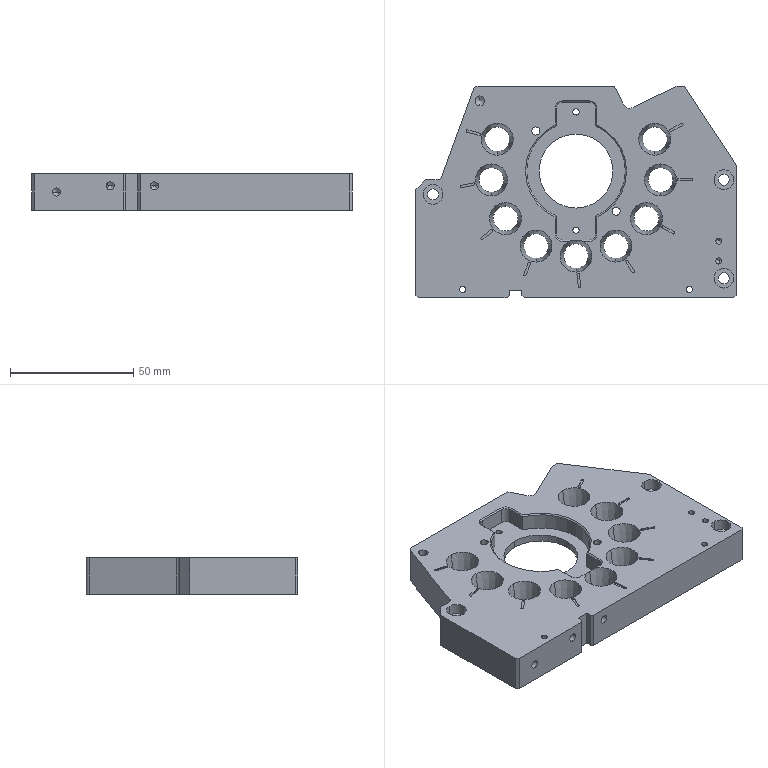NC program | NX | posted with a generic post | part box 130 x 86 x 15 mm
Lines 3061 to 5031 of 5031, first 1542 of 1963 lines:
(FLOOR_WALL_1_COPY_COPY , TOOL : D6JING)
N6120 T16 M6
N6122 G54
N6124 G17 G0 G90 X-5.595 Y18.197 B0. C0. S7500 M3
N6126 G43 Z30. H16
N6128 Z-3.9
N6130 G94 G1 X-9.7 Z-5. F1000.
N6132 X26.7 F1200.
N6134 Y15.397
N6136 X-9.7
N6138 Y12.597
N6140 X26.7
N6142 Y9.798
N6144 X-9.7
N6146 Y6.998
N6148 X26.7
N6150 Y4.198
N6152 X-9.7
N6154 Y1.398
N6156 X26.7
N6158 Y-1.401
N6160 X-9.7
N6162 Y-4.201
N6164 X26.7
N6166 Y-7.001
N6168 X-9.7
N6170 Y-9.801
N6172 X26.7
N6174 Y-12.6
N6176 X-9.7
N6178 Y-15.4
N6180 X26.7
N6182 Y-18.2
N6184 X-9.7
N6186 X-9.
N6188 X-10. F1000.
N6190 Y-18.5 F1200.
N6192 X27.
N6194 Y18.5
N6196 X-10.
N6198 Y-18.2
N6200 X-9.
N6202 Y-17.5
N6204 Z-4.
N6206 G0 Z30.
N6208 M5
(ZLEVEL_PROFILE_1_COPY_COPY , TOOL : D4)
N6210 T17 M6
N6212 G54
N6214 G17 G0 G90 X-10.2 Y-15.91 B0. C0. S6500 M3
N6216 G43 Z30. H17
N6218 Z-0.1
N6220 G94 G1 X-10.8 Y-16.257 F1650.
N6222 G3 X-11. Y-16.603 R0.4
N6224 G1 Y-19.
N6226 G3 X-10.5 Y-19.5 R0.5
N6228 G1 X-8.103
N6230 G3 X-7.757 Y-19.3 R0.4
N6232 G1 X-7.41 Y-18.7
N6234 G0 X-10.2 Y-15.91 Z-0.2
N6236 G1 X-10.8 Y-16.257
N6238 G3 X-11. Y-16.603 R0.4
N6240 G1 Y-19.
N6242 G3 X-10.5 Y-19.5 R0.5
N6244 G1 X-8.103
N6246 G3 X-7.757 Y-19.3 R0.4
N6248 G1 X-7.41 Y-18.7
N6250 G0 X-10.2 Y-15.91 Z-0.3
N6252 G1 X-10.8 Y-16.257
N6254 G3 X-11. Y-16.603 R0.4
N6256 G1 Y-19.
N6258 G3 X-10.5 Y-19.5 R0.5
N6260 G1 X-8.103
N6262 G3 X-7.757 Y-19.3 R0.4
N6264 G1 X-7.41 Y-18.7
N6266 G0 X-10.2 Y-15.91 Z-0.4
N6268 G1 X-10.8 Y-16.257
N6270 G3 X-11. Y-16.603 R0.4
N6272 G1 Y-19.
N6274 G3 X-10.5 Y-19.5 R0.5
N6276 G1 X-8.103
N6278 G3 X-7.757 Y-19.3 R0.4
N6280 G1 X-7.41 Y-18.7
N6282 G0 X-10.2 Y-15.91 Z-0.5
N6284 G1 X-10.8 Y-16.257
N6286 G3 X-11. Y-16.603 R0.4
N6288 G1 Y-19.
N6290 G3 X-10.5 Y-19.5 R0.5
N6292 G1 X-8.103
N6294 G3 X-7.757 Y-19.3 R0.4
N6296 G1 X-7.41 Y-18.7
N6298 G0 X-10.2 Y-15.91 Z-0.6
N6300 G1 X-10.8 Y-16.257
N6302 G3 X-11. Y-16.603 R0.4
N6304 G1 Y-19.
N6306 G3 X-10.5 Y-19.5 R0.5
N6308 G1 X-8.103
N6310 G3 X-7.757 Y-19.3 R0.4
N6312 G1 X-7.41 Y-18.7
N6314 G0 X-10.2 Y-15.91 Z-0.7
N6316 G1 X-10.8 Y-16.257
N6318 G3 X-11. Y-16.603 R0.4
N6320 G1 Y-19.
N6322 G3 X-10.5 Y-19.5 R0.5
N6324 G1 X-8.103
N6326 G3 X-7.757 Y-19.3 R0.4
N6328 G1 X-7.41 Y-18.7
N6330 G0 X-10.2 Y-15.91 Z-0.8
N6332 G1 X-10.8 Y-16.257
N6334 G3 X-11. Y-16.603 R0.4
N6336 G1 Y-19.
N6338 G3 X-10.5 Y-19.5 R0.5
N6340 G1 X-8.103
N6342 G3 X-7.757 Y-19.3 R0.4
N6344 G1 X-7.41 Y-18.7
N6346 G0 X-10.2 Y-15.91 Z-0.9
N6348 G1 X-10.8 Y-16.257
N6350 G3 X-11. Y-16.603 R0.4
N6352 G1 Y-19.
N6354 G3 X-10.5 Y-19.5 R0.5
N6356 G1 X-8.103
N6358 G3 X-7.757 Y-19.3 R0.4
N6360 G1 X-7.41 Y-18.7
N6362 G0 X-10.2 Y-15.91 Z-1.
N6364 G1 X-10.8 Y-16.257
N6366 G3 X-11. Y-16.603 R0.4
N6368 G1 Y-19.
N6370 G3 X-10.5 Y-19.5 R0.5
N6372 G1 X-8.103
N6374 G3 X-7.757 Y-19.3 R0.4
N6376 G1 X-7.41 Y-18.7
N6378 G0 X-10.2 Y-15.91 Z-1.1
N6380 G1 X-10.8 Y-16.257
N6382 G3 X-11. Y-16.603 R0.4
N6384 G1 Y-19.
N6386 G3 X-10.5 Y-19.5 R0.5
N6388 G1 X-8.103
N6390 G3 X-7.757 Y-19.3 R0.4
N6392 G1 X-7.41 Y-18.7
N6394 G0 X-10.2 Y-15.91 Z-1.2
N6396 G1 X-10.8 Y-16.257
N6398 G3 X-11. Y-16.603 R0.4
N6400 G1 Y-19.
N6402 G3 X-10.5 Y-19.5 R0.5
N6404 G1 X-8.103
N6406 G3 X-7.757 Y-19.3 R0.4
N6408 G1 X-7.41 Y-18.7
N6410 G0 X-10.2 Y-15.91 Z-1.3
N6412 G1 X-10.8 Y-16.257
N6414 G3 X-11. Y-16.603 R0.4
N6416 G1 Y-19.
N6418 G3 X-10.5 Y-19.5 R0.5
N6420 G1 X-8.103
N6422 G3 X-7.757 Y-19.3 R0.4
N6424 G1 X-7.41 Y-18.7
N6426 G0 X-10.2 Y-15.91 Z-1.4
N6428 G1 X-10.8 Y-16.257
N6430 G3 X-11. Y-16.603 R0.4
N6432 G1 Y-19.
N6434 G3 X-10.5 Y-19.5 R0.5
N6436 G1 X-8.103
N6438 G3 X-7.757 Y-19.3 R0.4
N6440 G1 X-7.41 Y-18.7
N6442 G0 X-10.2 Y-15.91 Z-1.5
N6444 G1 X-10.8 Y-16.257
N6446 G3 X-11. Y-16.603 R0.4
N6448 G1 Y-19.
N6450 G3 X-10.5 Y-19.5 R0.5
N6452 G1 X-8.103
N6454 G3 X-7.757 Y-19.3 R0.4
N6456 G1 X-7.41 Y-18.7
N6458 G0 X-10.2 Y-15.91 Z-1.6
N6460 G1 X-10.8 Y-16.257
N6462 G3 X-11. Y-16.603 R0.4
N6464 G1 Y-19.
N6466 G3 X-10.5 Y-19.5 R0.5
N6468 G1 X-8.103
N6470 G3 X-7.757 Y-19.3 R0.4
N6472 G1 X-7.41 Y-18.7
N6474 G0 X-10.2 Y-15.91 Z-1.7
N6476 G1 X-10.8 Y-16.257
N6478 G3 X-11. Y-16.603 R0.4
N6480 G1 Y-19.
N6482 G3 X-10.5 Y-19.5 R0.5
N6484 G1 X-8.103
N6486 G3 X-7.757 Y-19.3 R0.4
N6488 G1 X-7.41 Y-18.7
N6490 G0 X-10.2 Y-15.91 Z-1.8
N6492 G1 X-10.8 Y-16.257
N6494 G3 X-11. Y-16.603 R0.4
N6496 G1 Y-19.
N6498 G3 X-10.5 Y-19.5 R0.5
N6500 G1 X-8.103
N6502 G3 X-7.757 Y-19.3 R0.4
N6504 G1 X-7.41 Y-18.7
N6506 G0 X-10.2 Y-15.91 Z-1.9
N6508 G1 X-10.8 Y-16.257
N6510 G3 X-11. Y-16.603 R0.4
N6512 G1 Y-19.
N6514 G3 X-10.5 Y-19.5 R0.5
N6516 G1 X-8.103
N6518 G3 X-7.757 Y-19.3 R0.4
N6520 G1 X-7.41 Y-18.7
N6522 G0 X-10.2 Y-15.91 Z-2.
N6524 G1 X-10.8 Y-16.257
N6526 G3 X-11. Y-16.603 R0.4
N6528 G1 Y-19.
N6530 G3 X-10.5 Y-19.5 R0.5
N6532 G1 X-8.103
N6534 G3 X-7.757 Y-19.3 R0.4
N6536 G1 X-7.41 Y-18.7
N6538 G0 X-10.2 Y-15.91 Z-2.1
N6540 G1 X-10.8 Y-16.257
N6542 G3 X-11. Y-16.603 R0.4
N6544 G1 Y-19.
N6546 G3 X-10.5 Y-19.5 R0.5
N6548 G1 X-8.103
N6550 G3 X-7.757 Y-19.3 R0.4
N6552 G1 X-7.41 Y-18.7
N6554 G0 X-10.2 Y-15.91 Z-2.2
N6556 G1 X-10.8 Y-16.257
N6558 G3 X-11. Y-16.603 R0.4
N6560 G1 Y-19.
N6562 G3 X-10.5 Y-19.5 R0.5
N6564 G1 X-8.103
N6566 G3 X-7.757 Y-19.3 R0.4
N6568 G1 X-7.41 Y-18.7
N6570 G0 X-10.2 Y-15.91 Z-2.3
N6572 G1 X-10.8 Y-16.257
N6574 G3 X-11. Y-16.603 R0.4
N6576 G1 Y-19.
N6578 G3 X-10.5 Y-19.5 R0.5
N6580 G1 X-8.103
N6582 G3 X-7.757 Y-19.3 R0.4
N6584 G1 X-7.41 Y-18.7
N6586 G0 X-10.2 Y-15.91 Z-2.4
N6588 G1 X-10.8 Y-16.257
N6590 G3 X-11. Y-16.603 R0.4
N6592 G1 Y-19.
N6594 G3 X-10.5 Y-19.5 R0.5
N6596 G1 X-8.103
N6598 G3 X-7.757 Y-19.3 R0.4
N6600 G1 X-7.41 Y-18.7
N6602 G0 X-10.2 Y-15.91 Z-2.5
N6604 G1 X-10.8 Y-16.257
N6606 G3 X-11. Y-16.603 R0.4
N6608 G1 Y-19.
N6610 G3 X-10.5 Y-19.5 R0.5
N6612 G1 X-8.103
N6614 G3 X-7.757 Y-19.3 R0.4
N6616 G1 X-7.41 Y-18.7
N6618 G0 X-10.2 Y-15.91 Z-2.6
N6620 G1 X-10.8 Y-16.257
N6622 G3 X-11. Y-16.603 R0.4
N6624 G1 Y-19.
N6626 G3 X-10.5 Y-19.5 R0.5
N6628 G1 X-8.103
N6630 G3 X-7.757 Y-19.3 R0.4
N6632 G1 X-7.41 Y-18.7
N6634 G0 X-10.2 Y-15.91 Z-2.7
N6636 G1 X-10.8 Y-16.257
N6638 G3 X-11. Y-16.603 R0.4
N6640 G1 Y-19.
N6642 G3 X-10.5 Y-19.5 R0.5
N6644 G1 X-8.103
N6646 G3 X-7.757 Y-19.3 R0.4
N6648 G1 X-7.41 Y-18.7
N6650 G0 X-10.2 Y-15.91 Z-2.8
N6652 G1 X-10.8 Y-16.257
N6654 G3 X-11. Y-16.603 R0.4
N6656 G1 Y-19.
N6658 G3 X-10.5 Y-19.5 R0.5
N6660 G1 X-8.103
N6662 G3 X-7.757 Y-19.3 R0.4
N6664 G1 X-7.41 Y-18.7
N6666 G0 X-10.2 Y-15.91 Z-2.9
N6668 G1 X-10.8 Y-16.257
N6670 G3 X-11. Y-16.603 R0.4
N6672 G1 Y-19.
N6674 G3 X-10.5 Y-19.5 R0.5
N6676 G1 X-8.103
N6678 G3 X-7.757 Y-19.3 R0.4
N6680 G1 X-7.41 Y-18.7
N6682 G0 X-10.2 Y-15.91 Z-3.
N6684 G1 X-10.8 Y-16.257
N6686 G3 X-11. Y-16.603 R0.4
N6688 G1 Y-19.
N6690 G3 X-10.5 Y-19.5 R0.5
N6692 G1 X-8.103
N6694 G3 X-7.757 Y-19.3 R0.4
N6696 G1 X-7.41 Y-18.7
N6698 G0 X-10.2 Y-15.91 Z-3.1
N6700 G1 X-10.8 Y-16.257
N6702 G3 X-11. Y-16.603 R0.4
N6704 G1 Y-19.
N6706 G3 X-10.5 Y-19.5 R0.5
N6708 G1 X-8.103
N6710 G3 X-7.757 Y-19.3 R0.4
N6712 G1 X-7.41 Y-18.7
N6714 G0 X-10.2 Y-15.91 Z-3.2
N6716 G1 X-10.8 Y-16.257
N6718 G3 X-11. Y-16.603 R0.4
N6720 G1 Y-19.
N6722 G3 X-10.5 Y-19.5 R0.5
N6724 G1 X-8.103
N6726 G3 X-7.757 Y-19.3 R0.4
N6728 G1 X-7.41 Y-18.7
N6730 G0 X-10.2 Y-15.91 Z-3.3
N6732 G1 X-10.8 Y-16.257
N6734 G3 X-11. Y-16.603 R0.4
N6736 G1 Y-19.
N6738 G3 X-10.5 Y-19.5 R0.5
N6740 G1 X-8.103
N6742 G3 X-7.757 Y-19.3 R0.4
N6744 G1 X-7.41 Y-18.7
N6746 G0 X-10.2 Y-15.91 Z-3.4
N6748 G1 X-10.8 Y-16.257
N6750 G3 X-11. Y-16.603 R0.4
N6752 G1 Y-19.
N6754 G3 X-10.5 Y-19.5 R0.5
N6756 G1 X-8.103
N6758 G3 X-7.757 Y-19.3 R0.4
N6760 G1 X-7.41 Y-18.7
N6762 G0 X-10.2 Y-15.91 Z-3.5
N6764 G1 X-10.8 Y-16.257
N6766 G3 X-11. Y-16.603 R0.4
N6768 G1 Y-19.
N6770 G3 X-10.5 Y-19.5 R0.5
N6772 G1 X-8.103
N6774 G3 X-7.757 Y-19.3 R0.4
N6776 G1 X-7.41 Y-18.7
N6778 G0 X-10.2 Y-15.91 Z-3.6
N6780 G1 X-10.8 Y-16.257
N6782 G3 X-11. Y-16.603 R0.4
N6784 G1 Y-19.
N6786 G3 X-10.5 Y-19.5 R0.5
N6788 G1 X-8.103
N6790 G3 X-7.757 Y-19.3 R0.4
N6792 G1 X-7.41 Y-18.7
N6794 G0 X-10.2 Y-15.91 Z-3.7
N6796 G1 X-10.8 Y-16.257
N6798 G3 X-11. Y-16.603 R0.4
N6800 G1 Y-19.
N6802 G3 X-10.5 Y-19.5 R0.5
N6804 G1 X-8.103
N6806 G3 X-7.757 Y-19.3 R0.4
N6808 G1 X-7.41 Y-18.7
N6810 G0 X-10.2 Y-15.91 Z-3.8
N6812 G1 X-10.8 Y-16.257
N6814 G3 X-11. Y-16.603 R0.4
N6816 G1 Y-19.
N6818 G3 X-10.5 Y-19.5 R0.5
N6820 G1 X-8.103
N6822 G3 X-7.757 Y-19.3 R0.4
N6824 G1 X-7.41 Y-18.7
N6826 G0 X-10.2 Y-15.91 Z-3.9
N6828 G1 X-10.8 Y-16.257
N6830 G3 X-11. Y-16.603 R0.4
N6832 G1 Y-19.
N6834 G3 X-10.5 Y-19.5 R0.5
N6836 G1 X-8.103
N6838 G3 X-7.757 Y-19.3 R0.4
N6840 G1 X-7.41 Y-18.7
N6842 G0 X-10.2 Y-15.91 Z-4.
N6844 G1 X-10.8 Y-16.257
N6846 G3 X-11. Y-16.603 R0.4
N6848 G1 Y-19.
N6850 G3 X-10.5 Y-19.5 R0.5
N6852 G1 X-8.103
N6854 G3 X-7.757 Y-19.3 R0.4
N6856 G1 X-7.41 Y-18.7
N6858 G0 X-10.2 Y-15.91 Z-4.1
N6860 G1 X-10.8 Y-16.257
N6862 G3 X-11. Y-16.603 R0.4
N6864 G1 Y-19.
N6866 G3 X-10.5 Y-19.5 R0.5
N6868 G1 X-8.103
N6870 G3 X-7.757 Y-19.3 R0.4
N6872 G1 X-7.41 Y-18.7
N6874 G0 X-10.2 Y-15.91 Z-4.2
N6876 G1 X-10.8 Y-16.257
N6878 G3 X-11. Y-16.603 R0.4
N6880 G1 Y-19.
N6882 G3 X-10.5 Y-19.5 R0.5
N6884 G1 X-8.103
N6886 G3 X-7.757 Y-19.3 R0.4
N6888 G1 X-7.41 Y-18.7
N6890 G0 X-10.2 Y-15.91 Z-4.3
N6892 G1 X-10.8 Y-16.257
N6894 G3 X-11. Y-16.603 R0.4
N6896 G1 Y-19.
N6898 G3 X-10.5 Y-19.5 R0.5
N6900 G1 X-8.103
N6902 G3 X-7.757 Y-19.3 R0.4
N6904 G1 X-7.41 Y-18.7
N6906 G0 X-10.2 Y-15.91 Z-4.4
N6908 G1 X-10.8 Y-16.257
N6910 G3 X-11. Y-16.603 R0.4
N6912 G1 Y-19.
N6914 G3 X-10.5 Y-19.5 R0.5
N6916 G1 X-8.103
N6918 G3 X-7.757 Y-19.3 R0.4
N6920 G1 X-7.41 Y-18.7
N6922 G0 X-10.2 Y-15.91 Z-4.5
N6924 G1 X-10.8 Y-16.257
N6926 G3 X-11. Y-16.603 R0.4
N6928 G1 Y-19.
N6930 G3 X-10.5 Y-19.5 R0.5
N6932 G1 X-8.103
N6934 G3 X-7.757 Y-19.3 R0.4
N6936 G1 X-7.41 Y-18.7
N6938 G0 X-10.2 Y-15.91 Z-4.6
N6940 G1 X-10.8 Y-16.257
N6942 G3 X-11. Y-16.603 R0.4
N6944 G1 Y-19.
N6946 G3 X-10.5 Y-19.5 R0.5
N6948 G1 X-8.103
N6950 G3 X-7.757 Y-19.3 R0.4
N6952 G1 X-7.41 Y-18.7
N6954 G0 X-10.2 Y-15.91 Z-4.7
N6956 G1 X-10.8 Y-16.257
N6958 G3 X-11. Y-16.603 R0.4
N6960 G1 Y-19.
N6962 G3 X-10.5 Y-19.5 R0.5
N6964 G1 X-8.103
N6966 G3 X-7.757 Y-19.3 R0.4
N6968 G1 X-7.41 Y-18.7
N6970 G0 X-10.2 Y-15.91 Z-4.8
N6972 G1 X-10.8 Y-16.257
N6974 G3 X-11. Y-16.603 R0.4
N6976 G1 Y-19.
N6978 G3 X-10.5 Y-19.5 R0.5
N6980 G1 X-8.103
N6982 G3 X-7.757 Y-19.3 R0.4
N6984 G1 X-7.41 Y-18.7
N6986 G0 X-10.2 Y-15.91 Z-4.9
N6988 G1 X-10.8 Y-16.257
N6990 G3 X-11. Y-16.603 R0.4
N6992 G1 Y-19.
N6994 G3 X-10.5 Y-19.5 R0.5
N6996 G1 X-8.103
N6998 G3 X-7.757 Y-19.3 R0.4
N7000 G1 X-7.41 Y-18.7
N7002 G0 X-10.2 Y-15.91 Z-5.
N7004 G1 X-10.8 Y-16.257
N7006 G3 X-11. Y-16.603 R0.4
N7008 G1 Y-19.
N7010 G3 X-10.5 Y-19.5 R0.5
N7012 G1 X-8.103
N7014 G3 X-7.757 Y-19.3 R0.4
N7016 G1 X-7.41 Y-18.7
N7018 G0 Z30.
N7020 X24.41
N7022 Z-0.1
N7024 G1 X24.757 Y-19.3
N7026 G3 X25.103 Y-19.5 R0.4
N7028 G1 X27.5
N7030 G3 X28. Y-19. R0.5
N7032 G1 Y-16.603
N7034 G3 X27.8 Y-16.257 R0.4
N7036 G1 X27.2 Y-15.91
N7038 G0 X24.41 Y-18.7 Z-0.2
N7040 G1 X24.757 Y-19.3
N7042 G3 X25.103 Y-19.5 R0.4
N7044 G1 X27.5
N7046 G3 X28. Y-19. R0.5
N7048 G1 Y-16.603
N7050 G3 X27.8 Y-16.257 R0.4
N7052 G1 X27.2 Y-15.91
N7054 G0 X24.41 Y-18.7 Z-0.3
N7056 G1 X24.757 Y-19.3
N7058 G3 X25.103 Y-19.5 R0.4
N7060 G1 X27.5
N7062 G3 X28. Y-19. R0.5
N7064 G1 Y-16.603
N7066 G3 X27.8 Y-16.257 R0.4
N7068 G1 X27.2 Y-15.91
N7070 G0 X24.41 Y-18.7 Z-0.4
N7072 G1 X24.757 Y-19.3
N7074 G3 X25.103 Y-19.5 R0.4
N7076 G1 X27.5
N7078 G3 X28. Y-19. R0.5
N7080 G1 Y-16.603
N7082 G3 X27.8 Y-16.257 R0.4
N7084 G1 X27.2 Y-15.91
N7086 G0 X24.41 Y-18.7 Z-0.5
N7088 G1 X24.757 Y-19.3
N7090 G3 X25.103 Y-19.5 R0.4
N7092 G1 X27.5
N7094 G3 X28. Y-19. R0.5
N7096 G1 Y-16.603
N7098 G3 X27.8 Y-16.257 R0.4
N7100 G1 X27.2 Y-15.91
N7102 G0 X24.41 Y-18.7 Z-0.6
N7104 G1 X24.757 Y-19.3
N7106 G3 X25.103 Y-19.5 R0.4
N7108 G1 X27.5
N7110 G3 X28. Y-19. R0.5
N7112 G1 Y-16.603
N7114 G3 X27.8 Y-16.257 R0.4
N7116 G1 X27.2 Y-15.91
N7118 G0 X24.41 Y-18.7 Z-0.7
N7120 G1 X24.757 Y-19.3
N7122 G3 X25.103 Y-19.5 R0.4
N7124 G1 X27.5
N7126 G3 X28. Y-19. R0.5
N7128 G1 Y-16.603
N7130 G3 X27.8 Y-16.257 R0.4
N7132 G1 X27.2 Y-15.91
N7134 G0 X24.41 Y-18.7 Z-0.8
N7136 G1 X24.757 Y-19.3
N7138 G3 X25.103 Y-19.5 R0.4
N7140 G1 X27.5
N7142 G3 X28. Y-19. R0.5
N7144 G1 Y-16.603
N7146 G3 X27.8 Y-16.257 R0.4
N7148 G1 X27.2 Y-15.91
N7150 G0 X24.41 Y-18.7 Z-0.9
N7152 G1 X24.757 Y-19.3
N7154 G3 X25.103 Y-19.5 R0.4
N7156 G1 X27.5
N7158 G3 X28. Y-19. R0.5
N7160 G1 Y-16.603
N7162 G3 X27.8 Y-16.257 R0.4
N7164 G1 X27.2 Y-15.91
N7166 G0 X24.41 Y-18.7 Z-1.
N7168 G1 X24.757 Y-19.3
N7170 G3 X25.103 Y-19.5 R0.4
N7172 G1 X27.5
N7174 G3 X28. Y-19. R0.5
N7176 G1 Y-16.603
N7178 G3 X27.8 Y-16.257 R0.4
N7180 G1 X27.2 Y-15.91
N7182 G0 X24.41 Y-18.7 Z-1.1
N7184 G1 X24.757 Y-19.3
N7186 G3 X25.103 Y-19.5 R0.4
N7188 G1 X27.5
N7190 G3 X28. Y-19. R0.5
N7192 G1 Y-16.603
N7194 G3 X27.8 Y-16.257 R0.4
N7196 G1 X27.2 Y-15.91
N7198 G0 X24.41 Y-18.7 Z-1.2
N7200 G1 X24.757 Y-19.3
N7202 G3 X25.103 Y-19.5 R0.4
N7204 G1 X27.5
N7206 G3 X28. Y-19. R0.5
N7208 G1 Y-16.603
N7210 G3 X27.8 Y-16.257 R0.4
N7212 G1 X27.2 Y-15.91
N7214 G0 X24.41 Y-18.7 Z-1.3
N7216 G1 X24.757 Y-19.3
N7218 G3 X25.103 Y-19.5 R0.4
N7220 G1 X27.5
N7222 G3 X28. Y-19. R0.5
N7224 G1 Y-16.603
N7226 G3 X27.8 Y-16.257 R0.4
N7228 G1 X27.2 Y-15.91
N7230 G0 X24.41 Y-18.7 Z-1.4
N7232 G1 X24.757 Y-19.3
N7234 G3 X25.103 Y-19.5 R0.4
N7236 G1 X27.5
N7238 G3 X28. Y-19. R0.5
N7240 G1 Y-16.603
N7242 G3 X27.8 Y-16.257 R0.4
N7244 G1 X27.2 Y-15.91
N7246 G0 X24.41 Y-18.7 Z-1.5
N7248 G1 X24.757 Y-19.3
N7250 G3 X25.103 Y-19.5 R0.4
N7252 G1 X27.5
N7254 G3 X28. Y-19. R0.5
N7256 G1 Y-16.603
N7258 G3 X27.8 Y-16.257 R0.4
N7260 G1 X27.2 Y-15.91
N7262 G0 X24.41 Y-18.7 Z-1.6
N7264 G1 X24.757 Y-19.3
N7266 G3 X25.103 Y-19.5 R0.4
N7268 G1 X27.5
N7270 G3 X28. Y-19. R0.5
N7272 G1 Y-16.603
N7274 G3 X27.8 Y-16.257 R0.4
N7276 G1 X27.2 Y-15.91
N7278 G0 X24.41 Y-18.7 Z-1.7
N7280 G1 X24.757 Y-19.3
N7282 G3 X25.103 Y-19.5 R0.4
N7284 G1 X27.5
N7286 G3 X28. Y-19. R0.5
N7288 G1 Y-16.603
N7290 G3 X27.8 Y-16.257 R0.4
N7292 G1 X27.2 Y-15.91
N7294 G0 X24.41 Y-18.7 Z-1.8
N7296 G1 X24.757 Y-19.3
N7298 G3 X25.103 Y-19.5 R0.4
N7300 G1 X27.5
N7302 G3 X28. Y-19. R0.5
N7304 G1 Y-16.603
N7306 G3 X27.8 Y-16.257 R0.4
N7308 G1 X27.2 Y-15.91
N7310 G0 X24.41 Y-18.7 Z-1.9
N7312 G1 X24.757 Y-19.3
N7314 G3 X25.103 Y-19.5 R0.4
N7316 G1 X27.5
N7318 G3 X28. Y-19. R0.5
N7320 G1 Y-16.603
N7322 G3 X27.8 Y-16.257 R0.4
N7324 G1 X27.2 Y-15.91
N7326 G0 X24.41 Y-18.7 Z-2.
N7328 G1 X24.757 Y-19.3
N7330 G3 X25.103 Y-19.5 R0.4
N7332 G1 X27.5
N7334 G3 X28. Y-19. R0.5
N7336 G1 Y-16.603
N7338 G3 X27.8 Y-16.257 R0.4
N7340 G1 X27.2 Y-15.91
N7342 G0 X24.41 Y-18.7 Z-2.1
N7344 G1 X24.757 Y-19.3
N7346 G3 X25.103 Y-19.5 R0.4
N7348 G1 X27.5
N7350 G3 X28. Y-19. R0.5
N7352 G1 Y-16.603
N7354 G3 X27.8 Y-16.257 R0.4
N7356 G1 X27.2 Y-15.91
N7358 G0 X24.41 Y-18.7 Z-2.2
N7360 G1 X24.757 Y-19.3
N7362 G3 X25.103 Y-19.5 R0.4
N7364 G1 X27.5
N7366 G3 X28. Y-19. R0.5
N7368 G1 Y-16.603
N7370 G3 X27.8 Y-16.257 R0.4
N7372 G1 X27.2 Y-15.91
N7374 G0 X24.41 Y-18.7 Z-2.3
N7376 G1 X24.757 Y-19.3
N7378 G3 X25.103 Y-19.5 R0.4
N7380 G1 X27.5
N7382 G3 X28. Y-19. R0.5
N7384 G1 Y-16.603
N7386 G3 X27.8 Y-16.257 R0.4
N7388 G1 X27.2 Y-15.91
N7390 G0 X24.41 Y-18.7 Z-2.4
N7392 G1 X24.757 Y-19.3
N7394 G3 X25.103 Y-19.5 R0.4
N7396 G1 X27.5
N7398 G3 X28. Y-19. R0.5
N7400 G1 Y-16.603
N7402 G3 X27.8 Y-16.257 R0.4
N7404 G1 X27.2 Y-15.91
N7406 G0 X24.41 Y-18.7 Z-2.5
N7408 G1 X24.757 Y-19.3
N7410 G3 X25.103 Y-19.5 R0.4
N7412 G1 X27.5
N7414 G3 X28. Y-19. R0.5
N7416 G1 Y-16.603
N7418 G3 X27.8 Y-16.257 R0.4
N7420 G1 X27.2 Y-15.91
N7422 G0 X24.41 Y-18.7 Z-2.6
N7424 G1 X24.757 Y-19.3
N7426 G3 X25.103 Y-19.5 R0.4
N7428 G1 X27.5
N7430 G3 X28. Y-19. R0.5
N7432 G1 Y-16.603
N7434 G3 X27.8 Y-16.257 R0.4
N7436 G1 X27.2 Y-15.91
N7438 G0 X24.41 Y-18.7 Z-2.7
N7440 G1 X24.757 Y-19.3
N7442 G3 X25.103 Y-19.5 R0.4
N7444 G1 X27.5
N7446 G3 X28. Y-19. R0.5
N7448 G1 Y-16.603
N7450 G3 X27.8 Y-16.257 R0.4
N7452 G1 X27.2 Y-15.91
N7454 G0 X24.41 Y-18.7 Z-2.8
N7456 G1 X24.757 Y-19.3
N7458 G3 X25.103 Y-19.5 R0.4
N7460 G1 X27.5
N7462 G3 X28. Y-19. R0.5
N7464 G1 Y-16.603
N7466 G3 X27.8 Y-16.257 R0.4
N7468 G1 X27.2 Y-15.91
N7470 G0 X24.41 Y-18.7 Z-2.9
N7472 G1 X24.757 Y-19.3
N7474 G3 X25.103 Y-19.5 R0.4
N7476 G1 X27.5
N7478 G3 X28. Y-19. R0.5
N7480 G1 Y-16.603
N7482 G3 X27.8 Y-16.257 R0.4
N7484 G1 X27.2 Y-15.91
N7486 G0 X24.41 Y-18.7 Z-3.
N7488 G1 X24.757 Y-19.3
N7490 G3 X25.103 Y-19.5 R0.4
N7492 G1 X27.5
N7494 G3 X28. Y-19. R0.5
N7496 G1 Y-16.603
N7498 G3 X27.8 Y-16.257 R0.4
N7500 G1 X27.2 Y-15.91
N7502 G0 X24.41 Y-18.7 Z-3.1
N7504 G1 X24.757 Y-19.3
N7506 G3 X25.103 Y-19.5 R0.4
N7508 G1 X27.5
N7510 G3 X28. Y-19. R0.5
N7512 G1 Y-16.603
N7514 G3 X27.8 Y-16.257 R0.4
N7516 G1 X27.2 Y-15.91
N7518 G0 X24.41 Y-18.7 Z-3.2
N7520 G1 X24.757 Y-19.3
N7522 G3 X25.103 Y-19.5 R0.4
N7524 G1 X27.5
N7526 G3 X28. Y-19. R0.5
N7528 G1 Y-16.603
N7530 G3 X27.8 Y-16.257 R0.4
N7532 G1 X27.2 Y-15.91
N7534 G0 X24.41 Y-18.7 Z-3.3
N7536 G1 X24.757 Y-19.3
N7538 G3 X25.103 Y-19.5 R0.4
N7540 G1 X27.5
N7542 G3 X28. Y-19. R0.5
N7544 G1 Y-16.603
N7546 G3 X27.8 Y-16.257 R0.4
N7548 G1 X27.2 Y-15.91
N7550 G0 X24.41 Y-18.7 Z-3.4
N7552 G1 X24.757 Y-19.3
N7554 G3 X25.103 Y-19.5 R0.4
N7556 G1 X27.5
N7558 G3 X28. Y-19. R0.5
N7560 G1 Y-16.603
N7562 G3 X27.8 Y-16.257 R0.4
N7564 G1 X27.2 Y-15.91
N7566 G0 X24.41 Y-18.7 Z-3.5
N7568 G1 X24.757 Y-19.3
N7570 G3 X25.103 Y-19.5 R0.4
N7572 G1 X27.5
N7574 G3 X28. Y-19. R0.5
N7576 G1 Y-16.603
N7578 G3 X27.8 Y-16.257 R0.4
N7580 G1 X27.2 Y-15.91
N7582 G0 X24.41 Y-18.7 Z-3.6
N7584 G1 X24.757 Y-19.3
N7586 G3 X25.103 Y-19.5 R0.4
N7588 G1 X27.5
N7590 G3 X28. Y-19. R0.5
N7592 G1 Y-16.603
N7594 G3 X27.8 Y-16.257 R0.4
N7596 G1 X27.2 Y-15.91
N7598 G0 X24.41 Y-18.7 Z-3.7
N7600 G1 X24.757 Y-19.3
N7602 G3 X25.103 Y-19.5 R0.4
N7604 G1 X27.5
N7606 G3 X28. Y-19. R0.5
N7608 G1 Y-16.603
N7610 G3 X27.8 Y-16.257 R0.4
N7612 G1 X27.2 Y-15.91
N7614 G0 X24.41 Y-18.7 Z-3.8
N7616 G1 X24.757 Y-19.3
N7618 G3 X25.103 Y-19.5 R0.4
N7620 G1 X27.5
N7622 G3 X28. Y-19. R0.5
N7624 G1 Y-16.603
N7626 G3 X27.8 Y-16.257 R0.4
N7628 G1 X27.2 Y-15.91
N7630 G0 X24.41 Y-18.7 Z-3.9
N7632 G1 X24.757 Y-19.3
N7634 G3 X25.103 Y-19.5 R0.4
N7636 G1 X27.5
N7638 G3 X28. Y-19. R0.5
N7640 G1 Y-16.603
N7642 G3 X27.8 Y-16.257 R0.4
N7644 G1 X27.2 Y-15.91
N7646 G0 X24.41 Y-18.7 Z-4.
N7648 G1 X24.757 Y-19.3
N7650 G3 X25.103 Y-19.5 R0.4
N7652 G1 X27.5
N7654 G3 X28. Y-19. R0.5
N7656 G1 Y-16.603
N7658 G3 X27.8 Y-16.257 R0.4
N7660 G1 X27.2 Y-15.91
N7662 G0 X24.41 Y-18.7 Z-4.1
N7664 G1 X24.757 Y-19.3
N7666 G3 X25.103 Y-19.5 R0.4
N7668 G1 X27.5
N7670 G3 X28. Y-19. R0.5
N7672 G1 Y-16.603
N7674 G3 X27.8 Y-16.257 R0.4
N7676 G1 X27.2 Y-15.91
N7678 G0 X24.41 Y-18.7 Z-4.2
N7680 G1 X24.757 Y-19.3
N7682 G3 X25.103 Y-19.5 R0.4
N7684 G1 X27.5
N7686 G3 X28. Y-19. R0.5
N7688 G1 Y-16.603
N7690 G3 X27.8 Y-16.257 R0.4
N7692 G1 X27.2 Y-15.91
N7694 G0 X24.41 Y-18.7 Z-4.3
N7696 G1 X24.757 Y-19.3
N7698 G3 X25.103 Y-19.5 R0.4
N7700 G1 X27.5
N7702 G3 X28. Y-19. R0.5
N7704 G1 Y-16.603
N7706 G3 X27.8 Y-16.257 R0.4
N7708 G1 X27.2 Y-15.91
N7710 G0 X24.41 Y-18.7 Z-4.4
N7712 G1 X24.757 Y-19.3
N7714 G3 X25.103 Y-19.5 R0.4
N7716 G1 X27.5
N7718 G3 X28. Y-19. R0.5
N7720 G1 Y-16.603
N7722 G3 X27.8 Y-16.257 R0.4
N7724 G1 X27.2 Y-15.91
N7726 G0 X24.41 Y-18.7 Z-4.5
N7728 G1 X24.757 Y-19.3
N7730 G3 X25.103 Y-19.5 R0.4
N7732 G1 X27.5
N7734 G3 X28. Y-19. R0.5
N7736 G1 Y-16.603
N7738 G3 X27.8 Y-16.257 R0.4
N7740 G1 X27.2 Y-15.91
N7742 G0 X24.41 Y-18.7 Z-4.6
N7744 G1 X24.757 Y-19.3
N7746 G3 X25.103 Y-19.5 R0.4
N7748 G1 X27.5
N7750 G3 X28. Y-19. R0.5
N7752 G1 Y-16.603
N7754 G3 X27.8 Y-16.257 R0.4
N7756 G1 X27.2 Y-15.91
N7758 G0 X24.41 Y-18.7 Z-4.7
N7760 G1 X24.757 Y-19.3
N7762 G3 X25.103 Y-19.5 R0.4
N7764 G1 X27.5
N7766 G3 X28. Y-19. R0.5
N7768 G1 Y-16.603
N7770 G3 X27.8 Y-16.257 R0.4
N7772 G1 X27.2 Y-15.91
N7774 G0 X24.41 Y-18.7 Z-4.8
N7776 G1 X24.757 Y-19.3
N7778 G3 X25.103 Y-19.5 R0.4
N7780 G1 X27.5
N7782 G3 X28. Y-19. R0.5
N7784 G1 Y-16.603
N7786 G3 X27.8 Y-16.257 R0.4
N7788 G1 X27.2 Y-15.91
N7790 G0 X24.41 Y-18.7 Z-4.9
N7792 G1 X24.757 Y-19.3
N7794 G3 X25.103 Y-19.5 R0.4
N7796 G1 X27.5
N7798 G3 X28. Y-19. R0.5
N7800 G1 Y-16.603
N7802 G3 X27.8 Y-16.257 R0.4
N7804 G1 X27.2 Y-15.91
N7806 G0 X24.41 Y-18.7 Z-5.
N7808 G1 X24.757 Y-19.3
N7810 G3 X25.103 Y-19.5 R0.4
N7812 G1 X27.5
N7814 G3 X28. Y-19. R0.5
N7816 G1 Y-16.603
N7818 G3 X27.8 Y-16.257 R0.4
N7820 G1 X27.2 Y-15.91
N7822 G0 Z30.
N7824 Y15.91
N7826 Z-0.1
N7828 G1 X27.8 Y16.257
N7830 G3 X28. Y16.603 R0.4
N7832 G1 Y19.
N7834 G3 X27.5 Y19.5 R0.5
N7836 G1 X25.103
N7838 G3 X24.757 Y19.3 R0.4
N7840 G1 X24.41 Y18.7
N7842 G0 X27.2 Y15.91 Z-0.2
N7844 G1 X27.8 Y16.257
N7846 G3 X28. Y16.603 R0.4
N7848 G1 Y19.
N7850 G3 X27.5 Y19.5 R0.5
N7852 G1 X25.103
N7854 G3 X24.757 Y19.3 R0.4
N7856 G1 X24.41 Y18.7
N7858 G0 X27.2 Y15.91 Z-0.3
N7860 G1 X27.8 Y16.257
N7862 G3 X28. Y16.603 R0.4
N7864 G1 Y19.
N7866 G3 X27.5 Y19.5 R0.5
N7868 G1 X25.103
N7870 G3 X24.757 Y19.3 R0.4
N7872 G1 X24.41 Y18.7
N7874 G0 X27.2 Y15.91 Z-0.4
N7876 G1 X27.8 Y16.257
N7878 G3 X28. Y16.603 R0.4
N7880 G1 Y19.
N7882 G3 X27.5 Y19.5 R0.5
N7884 G1 X25.103
N7886 G3 X24.757 Y19.3 R0.4
N7888 G1 X24.41 Y18.7
N7890 G0 X27.2 Y15.91 Z-0.5
N7892 G1 X27.8 Y16.257
N7894 G3 X28. Y16.603 R0.4
N7896 G1 Y19.
N7898 G3 X27.5 Y19.5 R0.5
N7900 G1 X25.103
N7902 G3 X24.757 Y19.3 R0.4
N7904 G1 X24.41 Y18.7
N7906 G0 X27.2 Y15.91 Z-0.6
N7908 G1 X27.8 Y16.257
N7910 G3 X28. Y16.603 R0.4
N7912 G1 Y19.
N7914 G3 X27.5 Y19.5 R0.5
N7916 G1 X25.103
N7918 G3 X24.757 Y19.3 R0.4
N7920 G1 X24.41 Y18.7
N7922 G0 X27.2 Y15.91 Z-0.7
N7924 G1 X27.8 Y16.257
N7926 G3 X28. Y16.603 R0.4
N7928 G1 Y19.
N7930 G3 X27.5 Y19.5 R0.5
N7932 G1 X25.103
N7934 G3 X24.757 Y19.3 R0.4
N7936 G1 X24.41 Y18.7
N7938 G0 X27.2 Y15.91 Z-0.8
N7940 G1 X27.8 Y16.257
N7942 G3 X28. Y16.603 R0.4
N7944 G1 Y19.
N7946 G3 X27.5 Y19.5 R0.5
N7948 G1 X25.103
N7950 G3 X24.757 Y19.3 R0.4
N7952 G1 X24.41 Y18.7
N7954 G0 X27.2 Y15.91 Z-0.9
N7956 G1 X27.8 Y16.257
N7958 G3 X28. Y16.603 R0.4
N7960 G1 Y19.
N7962 G3 X27.5 Y19.5 R0.5
N7964 G1 X25.103
N7966 G3 X24.757 Y19.3 R0.4
N7968 G1 X24.41 Y18.7
N7970 G0 X27.2 Y15.91 Z-1.
N7972 G1 X27.8 Y16.257
N7974 G3 X28. Y16.603 R0.4
N7976 G1 Y19.
N7978 G3 X27.5 Y19.5 R0.5
N7980 G1 X25.103
N7982 G3 X24.757 Y19.3 R0.4
N7984 G1 X24.41 Y18.7
N7986 G0 X27.2 Y15.91 Z-1.1
N7988 G1 X27.8 Y16.257
N7990 G3 X28. Y16.603 R0.4
N7992 G1 Y19.
N7994 G3 X27.5 Y19.5 R0.5
N7996 G1 X25.103
N7998 G3 X24.757 Y19.3 R0.4
N8000 G1 X24.41 Y18.7
N8002 G0 X27.2 Y15.91 Z-1.2
N8004 G1 X27.8 Y16.257
N8006 G3 X28. Y16.603 R0.4
N8008 G1 Y19.
N8010 G3 X27.5 Y19.5 R0.5
N8012 G1 X25.103
N8014 G3 X24.757 Y19.3 R0.4
N8016 G1 X24.41 Y18.7
N8018 G0 X27.2 Y15.91 Z-1.3
N8020 G1 X27.8 Y16.257
N8022 G3 X28. Y16.603 R0.4
N8024 G1 Y19.
N8026 G3 X27.5 Y19.5 R0.5
N8028 G1 X25.103
N8030 G3 X24.757 Y19.3 R0.4
N8032 G1 X24.41 Y18.7
N8034 G0 X27.2 Y15.91 Z-1.4
N8036 G1 X27.8 Y16.257
N8038 G3 X28. Y16.603 R0.4
N8040 G1 Y19.
N8042 G3 X27.5 Y19.5 R0.5
N8044 G1 X25.103
N8046 G3 X24.757 Y19.3 R0.4
N8048 G1 X24.41 Y18.7
N8050 G0 X27.2 Y15.91 Z-1.5
N8052 G1 X27.8 Y16.257
N8054 G3 X28. Y16.603 R0.4
N8056 G1 Y19.
N8058 G3 X27.5 Y19.5 R0.5
N8060 G1 X25.103
N8062 G3 X24.757 Y19.3 R0.4
N8064 G1 X24.41 Y18.7
N8066 G0 X27.2 Y15.91 Z-1.6
N8068 G1 X27.8 Y16.257
N8070 G3 X28. Y16.603 R0.4
N8072 G1 Y19.
N8074 G3 X27.5 Y19.5 R0.5
N8076 G1 X25.103
N8078 G3 X24.757 Y19.3 R0.4
N8080 G1 X24.41 Y18.7
N8082 G0 X27.2 Y15.91 Z-1.7
N8084 G1 X27.8 Y16.257
N8086 G3 X28. Y16.603 R0.4
N8088 G1 Y19.
N8090 G3 X27.5 Y19.5 R0.5
N8092 G1 X25.103
N8094 G3 X24.757 Y19.3 R0.4
N8096 G1 X24.41 Y18.7
N8098 G0 X27.2 Y15.91 Z-1.8
N8100 G1 X27.8 Y16.257
N8102 G3 X28. Y16.603 R0.4
N8104 G1 Y19.
N8106 G3 X27.5 Y19.5 R0.5
N8108 G1 X25.103
N8110 G3 X24.757 Y19.3 R0.4
N8112 G1 X24.41 Y18.7
N8114 G0 X27.2 Y15.91 Z-1.9
N8116 G1 X27.8 Y16.257
N8118 G3 X28. Y16.603 R0.4
N8120 G1 Y19.
N8122 G3 X27.5 Y19.5 R0.5
N8124 G1 X25.103
N8126 G3 X24.757 Y19.3 R0.4
N8128 G1 X24.41 Y18.7
N8130 G0 X27.2 Y15.91 Z-2.
N8132 G1 X27.8 Y16.257
N8134 G3 X28. Y16.603 R0.4
N8136 G1 Y19.
N8138 G3 X27.5 Y19.5 R0.5
N8140 G1 X25.103
N8142 G3 X24.757 Y19.3 R0.4
N8144 G1 X24.41 Y18.7
N8146 G0 X27.2 Y15.91 Z-2.1
N8148 G1 X27.8 Y16.257
N8150 G3 X28. Y16.603 R0.4
N8152 G1 Y19.
N8154 G3 X27.5 Y19.5 R0.5
N8156 G1 X25.103
N8158 G3 X24.757 Y19.3 R0.4
N8160 G1 X24.41 Y18.7
N8162 G0 X27.2 Y15.91 Z-2.2
N8164 G1 X27.8 Y16.257
N8166 G3 X28. Y16.603 R0.4
N8168 G1 Y19.
N8170 G3 X27.5 Y19.5 R0.5
N8172 G1 X25.103
N8174 G3 X24.757 Y19.3 R0.4
N8176 G1 X24.41 Y18.7
N8178 G0 X27.2 Y15.91 Z-2.3
N8180 G1 X27.8 Y16.257
N8182 G3 X28. Y16.603 R0.4
N8184 G1 Y19.
N8186 G3 X27.5 Y19.5 R0.5
N8188 G1 X25.103
N8190 G3 X24.757 Y19.3 R0.4
N8192 G1 X24.41 Y18.7
N8194 G0 X27.2 Y15.91 Z-2.4
N8196 G1 X27.8 Y16.257
N8198 G3 X28. Y16.603 R0.4
N8200 G1 Y19.
N8202 G3 X27.5 Y19.5 R0.5
N8204 G1 X25.103
N8206 G3 X24.757 Y19.3 R0.4
N8208 G1 X24.41 Y18.7
N8210 G0 X27.2 Y15.91 Z-2.5
N8212 G1 X27.8 Y16.257
N8214 G3 X28. Y16.603 R0.4
N8216 G1 Y19.
N8218 G3 X27.5 Y19.5 R0.5
N8220 G1 X25.103
N8222 G3 X24.757 Y19.3 R0.4
N8224 G1 X24.41 Y18.7
N8226 G0 X27.2 Y15.91 Z-2.6
N8228 G1 X27.8 Y16.257
N8230 G3 X28. Y16.603 R0.4
N8232 G1 Y19.
N8234 G3 X27.5 Y19.5 R0.5
N8236 G1 X25.103
N8238 G3 X24.757 Y19.3 R0.4
N8240 G1 X24.41 Y18.7
N8242 G0 X27.2 Y15.91 Z-2.7
N8244 G1 X27.8 Y16.257
N8246 G3 X28. Y16.603 R0.4
N8248 G1 Y19.
N8250 G3 X27.5 Y19.5 R0.5
N8252 G1 X25.103
N8254 G3 X24.757 Y19.3 R0.4
N8256 G1 X24.41 Y18.7
N8258 G0 X27.2 Y15.91 Z-2.8
N8260 G1 X27.8 Y16.257
N8262 G3 X28. Y16.603 R0.4
N8264 G1 Y19.
N8266 G3 X27.5 Y19.5 R0.5
N8268 G1 X25.103
N8270 G3 X24.757 Y19.3 R0.4
N8272 G1 X24.41 Y18.7
N8274 G0 X27.2 Y15.91 Z-2.9
N8276 G1 X27.8 Y16.257
N8278 G3 X28. Y16.603 R0.4
N8280 G1 Y19.
N8282 G3 X27.5 Y19.5 R0.5
N8284 G1 X25.103
N8286 G3 X24.757 Y19.3 R0.4
N8288 G1 X24.41 Y18.7
N8290 G0 X27.2 Y15.91 Z-3.
N8292 G1 X27.8 Y16.257
N8294 G3 X28. Y16.603 R0.4
N8296 G1 Y19.
N8298 G3 X27.5 Y19.5 R0.5
N8300 G1 X25.103
N8302 G3 X24.757 Y19.3 R0.4
N8304 G1 X24.41 Y18.7
N8306 G0 X27.2 Y15.91 Z-3.1
N8308 G1 X27.8 Y16.257
N8310 G3 X28. Y16.603 R0.4
N8312 G1 Y19.
N8314 G3 X27.5 Y19.5 R0.5
N8316 G1 X25.103
N8318 G3 X24.757 Y19.3 R0.4
N8320 G1 X24.41 Y18.7
N8322 G0 X27.2 Y15.91 Z-3.2
N8324 G1 X27.8 Y16.257
N8326 G3 X28. Y16.603 R0.4
N8328 G1 Y19.
N8330 G3 X27.5 Y19.5 R0.5
N8332 G1 X25.103
N8334 G3 X24.757 Y19.3 R0.4
N8336 G1 X24.41 Y18.7
N8338 G0 X27.2 Y15.91 Z-3.3
N8340 G1 X27.8 Y16.257
N8342 G3 X28. Y16.603 R0.4
N8344 G1 Y19.
N8346 G3 X27.5 Y19.5 R0.5
N8348 G1 X25.103
N8350 G3 X24.757 Y19.3 R0.4
N8352 G1 X24.41 Y18.7
N8354 G0 X27.2 Y15.91 Z-3.4
N8356 G1 X27.8 Y16.257
N8358 G3 X28. Y16.603 R0.4
N8360 G1 Y19.
N8362 G3 X27.5 Y19.5 R0.5
N8364 G1 X25.103
N8366 G3 X24.757 Y19.3 R0.4
N8368 G1 X24.41 Y18.7
N8370 G0 X27.2 Y15.91 Z-3.5
N8372 G1 X27.8 Y16.257
N8374 G3 X28. Y16.603 R0.4
N8376 G1 Y19.
N8378 G3 X27.5 Y19.5 R0.5
N8380 G1 X25.103
N8382 G3 X24.757 Y19.3 R0.4
N8384 G1 X24.41 Y18.7
N8386 G0 X27.2 Y15.91 Z-3.6
N8388 G1 X27.8 Y16.257
N8390 G3 X28. Y16.603 R0.4
N8392 G1 Y19.
N8394 G3 X27.5 Y19.5 R0.5
N8396 G1 X25.103
N8398 G3 X24.757 Y19.3 R0.4
N8400 G1 X24.41 Y18.7
N8402 G0 X27.2 Y15.91 Z-3.7
N8404 G1 X27.8 Y16.257
N8406 G3 X28. Y16.603 R0.4
N8408 G1 Y19.
N8410 G3 X27.5 Y19.5 R0.5
N8412 G1 X25.103
N8414 G3 X24.757 Y19.3 R0.4
N8416 G1 X24.41 Y18.7
N8418 G0 X27.2 Y15.91 Z-3.8
N8420 G1 X27.8 Y16.257
N8422 G3 X28. Y16.603 R0.4
N8424 G1 Y19.
N8426 G3 X27.5 Y19.5 R0.5
N8428 G1 X25.103
N8430 G3 X24.757 Y19.3 R0.4
N8432 G1 X24.41 Y18.7
N8434 G0 X27.2 Y15.91 Z-3.9
N8436 G1 X27.8 Y16.257
N8438 G3 X28. Y16.603 R0.4
N8440 G1 Y19.
N8442 G3 X27.5 Y19.5 R0.5
N8444 G1 X25.103
N8446 G3 X24.757 Y19.3 R0.4
N8448 G1 X24.41 Y18.7
N8450 G0 X27.2 Y15.91 Z-4.
N8452 G1 X27.8 Y16.257
N8454 G3 X28. Y16.603 R0.4
N8456 G1 Y19.
N8458 G3 X27.5 Y19.5 R0.5
N8460 G1 X25.103
N8462 G3 X24.757 Y19.3 R0.4
N8464 G1 X24.41 Y18.7
N8466 G0 X27.2 Y15.91 Z-4.1
N8468 G1 X27.8 Y16.257
N8470 G3 X28. Y16.603 R0.4
N8472 G1 Y19.
N8474 G3 X27.5 Y19.5 R0.5
N8476 G1 X25.103
N8478 G3 X24.757 Y19.3 R0.4
N8480 G1 X24.41 Y18.7
N8482 G0 X27.2 Y15.91 Z-4.2
N8484 G1 X27.8 Y16.257
N8486 G3 X28. Y16.603 R0.4
N8488 G1 Y19.
N8490 G3 X27.5 Y19.5 R0.5
N8492 G1 X25.103
N8494 G3 X24.757 Y19.3 R0.4
N8496 G1 X24.41 Y18.7
N8498 G0 X27.2 Y15.91 Z-4.3
N8500 G1 X27.8 Y16.257
N8502 G3 X28. Y16.603 R0.4
N8504 G1 Y19.
N8506 G3 X27.5 Y19.5 R0.5
N8508 G1 X25.103
N8510 G3 X24.757 Y19.3 R0.4
N8512 G1 X24.41 Y18.7
N8514 G0 X27.2 Y15.91 Z-4.4
N8516 G1 X27.8 Y16.257
N8518 G3 X28. Y16.603 R0.4
N8520 G1 Y19.
N8522 G3 X27.5 Y19.5 R0.5
N8524 G1 X25.103
N8526 G3 X24.757 Y19.3 R0.4
N8528 G1 X24.41 Y18.7
N8530 G0 X27.2 Y15.91 Z-4.5
N8532 G1 X27.8 Y16.257
N8534 G3 X28. Y16.603 R0.4
N8536 G1 Y19.
N8538 G3 X27.5 Y19.5 R0.5
N8540 G1 X25.103
N8542 G3 X24.757 Y19.3 R0.4
N8544 G1 X24.41 Y18.7
N8546 G0 X27.2 Y15.91 Z-4.6
N8548 G1 X27.8 Y16.257
N8550 G3 X28. Y16.603 R0.4
N8552 G1 Y19.
N8554 G3 X27.5 Y19.5 R0.5
N8556 G1 X25.103
N8558 G3 X24.757 Y19.3 R0.4
N8560 G1 X24.41 Y18.7
N8562 G0 X27.2 Y15.91 Z-4.7
N8564 G1 X27.8 Y16.257
N8566 G3 X28. Y16.603 R0.4
N8568 G1 Y19.
N8570 G3 X27.5 Y19.5 R0.5
N8572 G1 X25.103
N8574 G3 X24.757 Y19.3 R0.4
N8576 G1 X24.41 Y18.7
N8578 G0 X27.2 Y15.91 Z-4.8
N8580 G1 X27.8 Y16.257
N8582 G3 X28. Y16.603 R0.4
N8584 G1 Y19.
N8586 G3 X27.5 Y19.5 R0.5
N8588 G1 X25.103
N8590 G3 X24.757 Y19.3 R0.4
N8592 G1 X24.41 Y18.7
N8594 G0 X27.2 Y15.91 Z-4.9
N8596 G1 X27.8 Y16.257
N8598 G3 X28. Y16.603 R0.4
N8600 G1 Y19.
N8602 G3 X27.5 Y19.5 R0.5
N8604 G1 X25.103
N8606 G3 X24.757 Y19.3 R0.4
N8608 G1 X24.41 Y18.7
N8610 G0 X27.2 Y15.91 Z-5.
N8612 G1 X27.8 Y16.257
N8614 G3 X28. Y16.603 R0.4
N8616 G1 Y19.
N8618 G3 X27.5 Y19.5 R0.5
N8620 G1 X25.103
N8622 G3 X24.757 Y19.3 R0.4
N8624 G1 X24.41 Y18.7
N8626 G0 Z30.
N8628 X-7.41
N8630 Z-0.1
N8632 G1 X-7.757 Y19.3
N8634 G3 X-8.103 Y19.5 R0.4
N8636 G1 X-10.5
N8638 G3 X-11. Y19. R0.5
N8640 G1 Y16.603
N8642 G3 X-10.8 Y16.257 R0.4
N8644 G1 X-10.2 Y15.91
N8646 G0 X-7.41 Y18.7 Z-0.2
N8648 G1 X-7.757 Y19.3
N8650 G3 X-8.103 Y19.5 R0.4
N8652 G1 X-10.5
N8654 G3 X-11. Y19. R0.5
N8656 G1 Y16.603
N8658 G3 X-10.8 Y16.257 R0.4
N8660 G1 X-10.2 Y15.91
N8662 G0 X-7.41 Y18.7 Z-0.3
N8664 G1 X-7.757 Y19.3
N8666 G3 X-8.103 Y19.5 R0.4
N8668 G1 X-10.5
N8670 G3 X-11. Y19. R0.5
N8672 G1 Y16.603
N8674 G3 X-10.8 Y16.257 R0.4
N8676 G1 X-10.2 Y15.91
N8678 G0 X-7.41 Y18.7 Z-0.4
N8680 G1 X-7.757 Y19.3
N8682 G3 X-8.103 Y19.5 R0.4
N8684 G1 X-10.5
N8686 G3 X-11. Y19. R0.5
N8688 G1 Y16.603
N8690 G3 X-10.8 Y16.257 R0.4
N8692 G1 X-10.2 Y15.91
N8694 G0 X-7.41 Y18.7 Z-0.5
N8696 G1 X-7.757 Y19.3
N8698 G3 X-8.103 Y19.5 R0.4
N8700 G1 X-10.5
N8702 G3 X-11. Y19. R0.5
N8704 G1 Y16.603
N8706 G3 X-10.8 Y16.257 R0.4
N8708 G1 X-10.2 Y15.91
N8710 G0 X-7.41 Y18.7 Z-0.6
N8712 G1 X-7.757 Y19.3
N8714 G3 X-8.103 Y19.5 R0.4
N8716 G1 X-10.5
N8718 G3 X-11. Y19. R0.5
N8720 G1 Y16.603
N8722 G3 X-10.8 Y16.257 R0.4
N8724 G1 X-10.2 Y15.91
N8726 G0 X-7.41 Y18.7 Z-0.7
N8728 G1 X-7.757 Y19.3
N8730 G3 X-8.103 Y19.5 R0.4
N8732 G1 X-10.5
N8734 G3 X-11. Y19. R0.5
N8736 G1 Y16.603
N8738 G3 X-10.8 Y16.257 R0.4
N8740 G1 X-10.2 Y15.91
N8742 G0 X-7.41 Y18.7 Z-0.8
N8744 G1 X-7.757 Y19.3
N8746 G3 X-8.103 Y19.5 R0.4
N8748 G1 X-10.5
N8750 G3 X-11. Y19. R0.5
N8752 G1 Y16.603
N8754 G3 X-10.8 Y16.257 R0.4
N8756 G1 X-10.2 Y15.91
N8758 G0 X-7.41 Y18.7 Z-0.9
N8760 G1 X-7.757 Y19.3
N8762 G3 X-8.103 Y19.5 R0.4
N8764 G1 X-10.5
N8766 G3 X-11. Y19. R0.5
N8768 G1 Y16.603
N8770 G3 X-10.8 Y16.257 R0.4
N8772 G1 X-10.2 Y15.91
N8774 G0 X-7.41 Y18.7 Z-1.
N8776 G1 X-7.757 Y19.3
N8778 G3 X-8.103 Y19.5 R0.4
N8780 G1 X-10.5
N8782 G3 X-11. Y19. R0.5
N8784 G1 Y16.603
N8786 G3 X-10.8 Y16.257 R0.4
N8788 G1 X-10.2 Y15.91
N8790 G0 X-7.41 Y18.7 Z-1.1
N8792 G1 X-7.757 Y19.3
N8794 G3 X-8.103 Y19.5 R0.4
N8796 G1 X-10.5
N8798 G3 X-11. Y19. R0.5
N8800 G1 Y16.603
N8802 G3 X-10.8 Y16.257 R0.4
N8804 G1 X-10.2 Y15.91
N8806 G0 X-7.41 Y18.7 Z-1.2
N8808 G1 X-7.757 Y19.3
N8810 G3 X-8.103 Y19.5 R0.4
N8812 G1 X-10.5
N8814 G3 X-11. Y19. R0.5
N8816 G1 Y16.603
N8818 G3 X-10.8 Y16.257 R0.4
N8820 G1 X-10.2 Y15.91
N8822 G0 X-7.41 Y18.7 Z-1.3
N8824 G1 X-7.757 Y19.3
N8826 G3 X-8.103 Y19.5 R0.4
N8828 G1 X-10.5
N8830 G3 X-11. Y19. R0.5
N8832 G1 Y16.603
N8834 G3 X-10.8 Y16.257 R0.4
N8836 G1 X-10.2 Y15.91
N8838 G0 X-7.41 Y18.7 Z-1.4
N8840 G1 X-7.757 Y19.3
N8842 G3 X-8.103 Y19.5 R0.4
N8844 G1 X-10.5
N8846 G3 X-11. Y19. R0.5
N8848 G1 Y16.603
N8850 G3 X-10.8 Y16.257 R0.4
N8852 G1 X-10.2 Y15.91
N8854 G0 X-7.41 Y18.7 Z-1.5
N8856 G1 X-7.757 Y19.3
N8858 G3 X-8.103 Y19.5 R0.4
N8860 G1 X-10.5
N8862 G3 X-11. Y19. R0.5
N8864 G1 Y16.603
N8866 G3 X-10.8 Y16.257 R0.4
N8868 G1 X-10.2 Y15.91
N8870 G0 X-7.41 Y18.7 Z-1.6
N8872 G1 X-7.757 Y19.3
N8874 G3 X-8.103 Y19.5 R0.4
N8876 G1 X-10.5
N8878 G3 X-11. Y19. R0.5
N8880 G1 Y16.603
N8882 G3 X-10.8 Y16.257 R0.4
N8884 G1 X-10.2 Y15.91
N8886 G0 X-7.41 Y18.7 Z-1.7
N8888 G1 X-7.757 Y19.3
N8890 G3 X-8.103 Y19.5 R0.4
N8892 G1 X-10.5
N8894 G3 X-11. Y19. R0.5
N8896 G1 Y16.603
N8898 G3 X-10.8 Y16.257 R0.4
N8900 G1 X-10.2 Y15.91
N8902 G0 X-7.41 Y18.7 Z-1.8
N8904 G1 X-7.757 Y19.3
N8906 G3 X-8.103 Y19.5 R0.4
N8908 G1 X-10.5
N8910 G3 X-11. Y19. R0.5
N8912 G1 Y16.603
N8914 G3 X-10.8 Y16.257 R0.4
N8916 G1 X-10.2 Y15.91
N8918 G0 X-7.41 Y18.7 Z-1.9
N8920 G1 X-7.757 Y19.3
N8922 G3 X-8.103 Y19.5 R0.4
N8924 G1 X-10.5
N8926 G3 X-11. Y19. R0.5
N8928 G1 Y16.603
N8930 G3 X-10.8 Y16.257 R0.4
N8932 G1 X-10.2 Y15.91
N8934 G0 X-7.41 Y18.7 Z-2.
N8936 G1 X-7.757 Y19.3
N8938 G3 X-8.103 Y19.5 R0.4
N8940 G1 X-10.5
N8942 G3 X-11. Y19. R0.5
N8944 G1 Y16.603
N8946 G3 X-10.8 Y16.257 R0.4
N8948 G1 X-10.2 Y15.91
N8950 G0 X-7.41 Y18.7 Z-2.1
N8952 G1 X-7.757 Y19.3
N8954 G3 X-8.103 Y19.5 R0.4
N8956 G1 X-10.5
N8958 G3 X-11. Y19. R0.5
N8960 G1 Y16.603
N8962 G3 X-10.8 Y16.257 R0.4
N8964 G1 X-10.2 Y15.91
N8966 G0 X-7.41 Y18.7 Z-2.2
N8968 G1 X-7.757 Y19.3
N8970 G3 X-8.103 Y19.5 R0.4
N8972 G1 X-10.5
N8974 G3 X-11. Y19. R0.5
N8976 G1 Y16.603
N8978 G3 X-10.8 Y16.257 R0.4
N8980 G1 X-10.2 Y15.91
N8982 G0 X-7.41 Y18.7 Z-2.3
N8984 G1 X-7.757 Y19.3
N8986 G3 X-8.103 Y19.5 R0.4
N8988 G1 X-10.5
N8990 G3 X-11. Y19. R0.5
N8992 G1 Y16.603
N8994 G3 X-10.8 Y16.257 R0.4
N8996 G1 X-10.2 Y15.91
N8998 G0 X-7.41 Y18.7 Z-2.4
N9000 G1 X-7.757 Y19.3
N9002 G3 X-8.103 Y19.5 R0.4
N9004 G1 X-10.5
N9006 G3 X-11. Y19. R0.5
N9008 G1 Y16.603
N9010 G3 X-10.8 Y16.257 R0.4
N9012 G1 X-10.2 Y15.91
N9014 G0 X-7.41 Y18.7 Z-2.5
N9016 G1 X-7.757 Y19.3
N9018 G3 X-8.103 Y19.5 R0.4
N9020 G1 X-10.5
N9022 G3 X-11. Y19. R0.5
N9024 G1 Y16.603
N9026 G3 X-10.8 Y16.257 R0.4
N9028 G1 X-10.2 Y15.91
N9030 G0 X-7.41 Y18.7 Z-2.6
N9032 G1 X-7.757 Y19.3
N9034 G3 X-8.103 Y19.5 R0.4
N9036 G1 X-10.5
N9038 G3 X-11. Y19. R0.5
N9040 G1 Y16.603
N9042 G3 X-10.8 Y16.257 R0.4
N9044 G1 X-10.2 Y15.91
N9046 G0 X-7.41 Y18.7 Z-2.7
N9048 G1 X-7.757 Y19.3
N9050 G3 X-8.103 Y19.5 R0.4
N9052 G1 X-10.5
N9054 G3 X-11. Y19. R0.5
N9056 G1 Y16.603
N9058 G3 X-10.8 Y16.257 R0.4
N9060 G1 X-10.2 Y15.91
N9062 G0 X-7.41 Y18.7 Z-2.8
N9064 G1 X-7.757 Y19.3
N9066 G3 X-8.103 Y19.5 R0.4
N9068 G1 X-10.5
N9070 G3 X-11. Y19. R0.5
N9072 G1 Y16.603
N9074 G3 X-10.8 Y16.257 R0.4
N9076 G1 X-10.2 Y15.91
N9078 G0 X-7.41 Y18.7 Z-2.9
N9080 G1 X-7.757 Y19.3
N9082 G3 X-8.103 Y19.5 R0.4
N9084 G1 X-10.5
N9086 G3 X-11. Y19. R0.5
N9088 G1 Y16.603
N9090 G3 X-10.8 Y16.257 R0.4
N9092 G1 X-10.2 Y15.91
N9094 G0 X-7.41 Y18.7 Z-3.
N9096 G1 X-7.757 Y19.3
N9098 G3 X-8.103 Y19.5 R0.4
N9100 G1 X-10.5
N9102 G3 X-11. Y19. R0.5
N9104 G1 Y16.603
N9106 G3 X-10.8 Y16.257 R0.4
N9108 G1 X-10.2 Y15.91
N9110 G0 X-7.41 Y18.7 Z-3.1
N9112 G1 X-7.757 Y19.3
N9114 G3 X-8.103 Y19.5 R0.4
N9116 G1 X-10.5
N9118 G3 X-11. Y19. R0.5
N9120 G1 Y16.603
N9122 G3 X-10.8 Y16.257 R0.4
N9124 G1 X-10.2 Y15.91
N9126 G0 X-7.41 Y18.7 Z-3.2
N9128 G1 X-7.757 Y19.3
N9130 G3 X-8.103 Y19.5 R0.4
N9132 G1 X-10.5
N9134 G3 X-11. Y19. R0.5
N9136 G1 Y16.603
N9138 G3 X-10.8 Y16.257 R0.4
N9140 G1 X-10.2 Y15.91
N9142 G0 X-7.41 Y18.7 Z-3.3
N9144 G1 X-7.757 Y19.3
N9146 G3 X-8.103 Y19.5 R0.4
N9148 G1 X-10.5
N9150 G3 X-11. Y19. R0.5
N9152 G1 Y16.603
N9154 G3 X-10.8 Y16.257 R0.4
N9156 G1 X-10.2 Y15.91
N9158 G0 X-7.41 Y18.7 Z-3.4
N9160 G1 X-7.757 Y19.3
N9162 G3 X-8.103 Y19.5 R0.4
N9164 G1 X-10.5
N9166 G3 X-11. Y19. R0.5
N9168 G1 Y16.603
N9170 G3 X-10.8 Y16.257 R0.4
N9172 G1 X-10.2 Y15.91
N9174 G0 X-7.41 Y18.7 Z-3.5
N9176 G1 X-7.757 Y19.3
N9178 G3 X-8.103 Y19.5 R0.4
N9180 G1 X-10.5
N9182 G3 X-11. Y19. R0.5
N9184 G1 Y16.603
N9186 G3 X-10.8 Y16.257 R0.4
N9188 G1 X-10.2 Y15.91
N9190 G0 X-7.41 Y18.7 Z-3.6
N9192 G1 X-7.757 Y19.3
N9194 G3 X-8.103 Y19.5 R0.4
N9196 G1 X-10.5
N9198 G3 X-11. Y19. R0.5